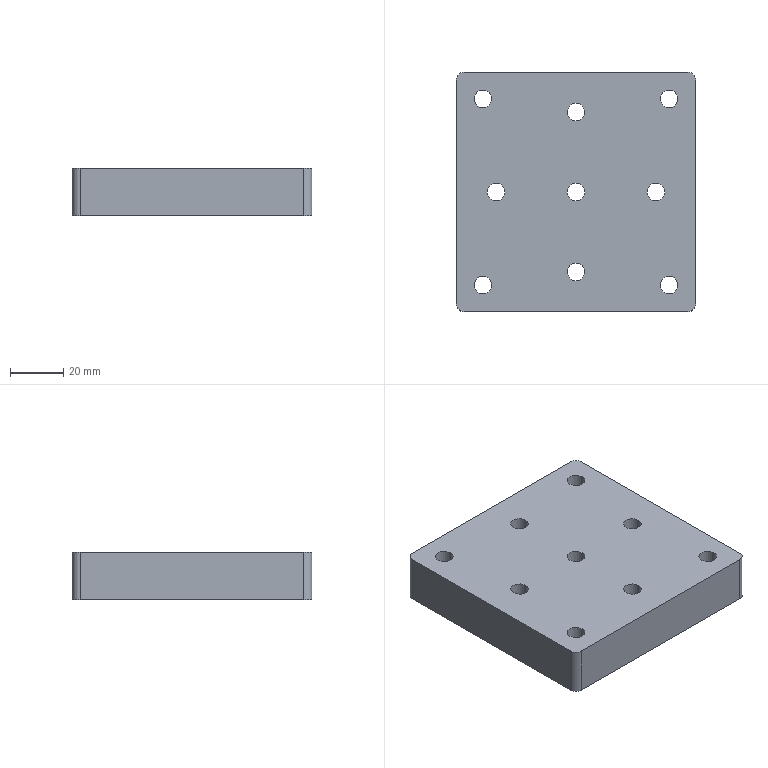Part | NX | features BREP 1 | 1 solid | 43 faces | box 90 x 90 x 18 mm | volume 136139 mm3 | cylinder 32 | plane 11 | commonest cylinder face diameters 6.6 x10 12 x10 6.647 x8 6 x4
STEP:
#1=CARTESIAN_POINT('',(6.,-30.,10.));
#2=VERTEX_POINT('',#1);
#3=CARTESIAN_POINT('',(-6.,-30.,10.));
#4=VERTEX_POINT('',#3);
#5=CARTESIAN_POINT('',(0.,-30.,10.));
#6=DIRECTION('',(0.,0.,-1.));
#7=DIRECTION('',(1.,0.,0.));
#8=AXIS2_PLACEMENT_3D('',#5,#6,#7);
#9=CIRCLE('',#8,6.);
#10=EDGE_CURVE('',#2,#4,#9,.T.);
#11=ORIENTED_EDGE('',*,*,#10,.T.);
#12=CARTESIAN_POINT('',(0.,-30.,10.));
#13=DIRECTION('',(0.,0.,-1.));
#14=DIRECTION('',(-1.,0.,0.));
#15=AXIS2_PLACEMENT_3D('',#12,#13,#14);
#16=CIRCLE('',#15,6.);
#17=EDGE_CURVE('',#4,#2,#16,.T.);
#18=ORIENTED_EDGE('',*,*,#17,.T.);
#19=EDGE_LOOP('',(#11,#18));
#20=FACE_BOUND('',#19,.T.);
#21=CARTESIAN_POINT('',(3.3,-30.,10.));
#22=VERTEX_POINT('',#21);
#23=CARTESIAN_POINT('',(-3.3,-30.,10.));
#24=VERTEX_POINT('',#23);
#25=CARTESIAN_POINT('',(0.,-30.,10.));
#26=DIRECTION('',(0.,0.,1.));
#27=DIRECTION('',(1.,0.,0.));
#28=AXIS2_PLACEMENT_3D('',#25,#26,#27);
#29=CIRCLE('',#28,3.3);
#30=EDGE_CURVE('',#22,#24,#29,.T.);
#31=ORIENTED_EDGE('',*,*,#30,.T.);
#32=CARTESIAN_POINT('',(0.,-30.,10.));
#33=DIRECTION('',(0.,0.,1.));
#34=DIRECTION('',(-1.,0.,0.));
#35=AXIS2_PLACEMENT_3D('',#32,#33,#34);
#36=CIRCLE('',#35,3.3);
#37=EDGE_CURVE('',#24,#22,#36,.T.);
#38=ORIENTED_EDGE('',*,*,#37,.T.);
#39=EDGE_LOOP('',(#31,#38));
#40=FACE_BOUND('',#39,.T.);
#41=CARTESIAN_POINT('',(3.3,-30.,10.));
#42=DIRECTION('',(0.,0.,1.));
#43=DIRECTION('',(1.,0.,0.));
#44=AXIS2_PLACEMENT_3D('',#41,#42,#43);
#45=PLANE('',#44);
#46=ADVANCED_FACE('',(#20,#40),#45,.F.);
#47=CARTESIAN_POINT('',(6.,-30.,0.));
#48=VERTEX_POINT('',#47);
#49=CARTESIAN_POINT('',(6.,-30.,0.));
#50=DIRECTION('',(0.,0.,1.));
#51=VECTOR('',#50,1000.);
#52=LINE('',#49,#51);
#53=EDGE_CURVE('',#2,#48,#52,.F.);
#54=ORIENTED_EDGE('',*,*,#53,.F.);
#55=ORIENTED_EDGE('',*,*,#17,.F.);
#56=CARTESIAN_POINT('',(-6.,-30.,0.));
#57=VERTEX_POINT('',#56);
#58=CARTESIAN_POINT('',(-6.,-30.,0.));
#59=DIRECTION('',(0.,0.,1.));
#60=VECTOR('',#59,1000.);
#61=LINE('',#58,#60);
#62=EDGE_CURVE('',#4,#57,#61,.F.);
#63=ORIENTED_EDGE('',*,*,#62,.T.);
#64=CARTESIAN_POINT('',(0.,-30.,0.));
#65=DIRECTION('',(0.,0.,1.));
#66=DIRECTION('',(1.,0.,0.));
#67=AXIS2_PLACEMENT_3D('',#64,#65,#66);
#68=CIRCLE('',#67,6.);
#69=EDGE_CURVE('',#48,#57,#68,.T.);
#70=ORIENTED_EDGE('',*,*,#69,.F.);
#71=EDGE_LOOP('',(#54,#55,#63,#70));
#72=FACE_BOUND('',#71,.T.);
#73=CARTESIAN_POINT('',(0.,-30.,0.));
#74=DIRECTION('',(0.,0.,1.));
#75=DIRECTION('',(-1.,0.,0.));
#76=AXIS2_PLACEMENT_3D('',#73,#74,#75);
#77=CYLINDRICAL_SURFACE('',#76,6.);
#78=ADVANCED_FACE('',(#72),#77,.F.);
#79=CARTESIAN_POINT('',(-42.,45.,0.));
#80=VERTEX_POINT('',#79);
#81=CARTESIAN_POINT('',(42.,45.,0.));
#82=VERTEX_POINT('',#81);
#83=CARTESIAN_POINT('',(-42.,45.,0.));
#84=DIRECTION('',(1.,0.,0.));
#85=VECTOR('',#84,1000.);
#86=LINE('',#83,#85);
#87=EDGE_CURVE('',#80,#82,#86,.T.);
#88=ORIENTED_EDGE('',*,*,#87,.T.);
#89=CARTESIAN_POINT('',(45.,42.,0.));
#90=VERTEX_POINT('',#89);
#91=CARTESIAN_POINT('',(42.,42.,0.));
#92=DIRECTION('',(0.,0.,-1.));
#93=DIRECTION('',(0.,1.,0.));
#94=AXIS2_PLACEMENT_3D('',#91,#92,#93);
#95=CIRCLE('',#94,3.);
#96=EDGE_CURVE('',#82,#90,#95,.T.);
#97=ORIENTED_EDGE('',*,*,#96,.T.);
#98=CARTESIAN_POINT('',(45.,-42.,0.));
#99=VERTEX_POINT('',#98);
#100=CARTESIAN_POINT('',(45.,42.,0.));
#101=DIRECTION('',(0.,-1.,0.));
#102=VECTOR('',#101,1000.);
#103=LINE('',#100,#102);
#104=EDGE_CURVE('',#90,#99,#103,.T.);
#105=ORIENTED_EDGE('',*,*,#104,.T.);
#106=CARTESIAN_POINT('',(42.,-45.,0.));
#107=VERTEX_POINT('',#106);
#108=CARTESIAN_POINT('',(42.,-42.,0.));
#109=DIRECTION('',(0.,0.,-1.));
#110=DIRECTION('',(1.,0.,0.));
#111=AXIS2_PLACEMENT_3D('',#108,#109,#110);
#112=CIRCLE('',#111,3.);
#113=EDGE_CURVE('',#99,#107,#112,.T.);
#114=ORIENTED_EDGE('',*,*,#113,.T.);
#115=CARTESIAN_POINT('',(-42.,-45.,0.));
#116=VERTEX_POINT('',#115);
#117=CARTESIAN_POINT('',(42.,-45.,0.));
#118=DIRECTION('',(-1.,0.,0.));
#119=VECTOR('',#118,1000.);
#120=LINE('',#117,#119);
#121=EDGE_CURVE('',#107,#116,#120,.T.);
#122=ORIENTED_EDGE('',*,*,#121,.T.);
#123=CARTESIAN_POINT('',(-45.,-42.,0.));
#124=VERTEX_POINT('',#123);
#125=CARTESIAN_POINT('',(-42.,-42.,0.));
#126=DIRECTION('',(0.,0.,-1.));
#127=DIRECTION('',(0.,-1.,0.));
#128=AXIS2_PLACEMENT_3D('',#125,#126,#127);
#129=CIRCLE('',#128,3.);
#130=EDGE_CURVE('',#116,#124,#129,.T.);
#131=ORIENTED_EDGE('',*,*,#130,.T.);
#132=CARTESIAN_POINT('',(-45.,42.,0.));
#133=VERTEX_POINT('',#132);
#134=CARTESIAN_POINT('',(-45.,-42.,0.));
#135=DIRECTION('',(0.,1.,0.));
#136=VECTOR('',#135,1000.);
#137=LINE('',#134,#136);
#138=EDGE_CURVE('',#124,#133,#137,.T.);
#139=ORIENTED_EDGE('',*,*,#138,.T.);
#140=CARTESIAN_POINT('',(-42.,42.,0.));
#141=DIRECTION('',(0.,0.,-1.));
#142=DIRECTION('',(-1.,0.,0.));
#143=AXIS2_PLACEMENT_3D('',#140,#141,#142);
#144=CIRCLE('',#143,3.);
#145=EDGE_CURVE('',#133,#80,#144,.T.);
#146=ORIENTED_EDGE('',*,*,#145,.T.);
#147=EDGE_LOOP('',(#88,#97,#105,#114,#122,#131,#139,#146));
#148=FACE_BOUND('',#147,.T.);
#149=CARTESIAN_POINT('',(-6.,0.,0.));
#150=VERTEX_POINT('',#149);
#151=CARTESIAN_POINT('',(6.,0.,0.));
#152=VERTEX_POINT('',#151);
#153=CARTESIAN_POINT('',(0.,0.,0.));
#154=DIRECTION('',(0.,0.,1.));
#155=DIRECTION('',(-1.,0.,0.));
#156=AXIS2_PLACEMENT_3D('',#153,#154,#155);
#157=CIRCLE('',#156,6.);
#158=EDGE_CURVE('',#150,#152,#157,.T.);
#159=ORIENTED_EDGE('',*,*,#158,.T.);
#160=CARTESIAN_POINT('',(0.,0.,0.));
#161=DIRECTION('',(0.,0.,1.));
#162=DIRECTION('',(1.,0.,0.));
#163=AXIS2_PLACEMENT_3D('',#160,#161,#162);
#164=CIRCLE('',#163,6.);
#165=EDGE_CURVE('',#152,#150,#164,.T.);
#166=ORIENTED_EDGE('',*,*,#165,.T.);
#167=EDGE_LOOP('',(#159,#166));
#168=FACE_BOUND('',#167,.T.);
#169=ORIENTED_EDGE('',*,*,#69,.T.);
#170=CARTESIAN_POINT('',(0.,-30.,0.));
#171=DIRECTION('',(0.,0.,1.));
#172=DIRECTION('',(-1.,0.,0.));
#173=AXIS2_PLACEMENT_3D('',#170,#171,#172);
#174=CIRCLE('',#173,6.);
#175=EDGE_CURVE('',#57,#48,#174,.T.);
#176=ORIENTED_EDGE('',*,*,#175,.T.);
#177=EDGE_LOOP('',(#169,#176));
#178=FACE_BOUND('',#177,.T.);
#179=CARTESIAN_POINT('',(-31.677,35.,0.));
#180=VERTEX_POINT('',#179);
#181=CARTESIAN_POINT('',(-38.324,35.,0.));
#182=VERTEX_POINT('',#181);
#183=CARTESIAN_POINT('',(-35.,35.,0.));
#184=DIRECTION('',(0.,0.,1.));
#185=DIRECTION('',(1.,0.,0.));
#186=AXIS2_PLACEMENT_3D('',#183,#184,#185);
#187=CIRCLE('',#186,3.324);
#188=EDGE_CURVE('',#180,#182,#187,.T.);
#189=ORIENTED_EDGE('',*,*,#188,.T.);
#190=CARTESIAN_POINT('',(-35.,35.,0.));
#191=DIRECTION('',(0.,0.,1.));
#192=DIRECTION('',(-1.,0.,0.));
#193=AXIS2_PLACEMENT_3D('',#190,#191,#192);
#194=CIRCLE('',#193,3.324);
#195=EDGE_CURVE('',#182,#180,#194,.T.);
#196=ORIENTED_EDGE('',*,*,#195,.T.);
#197=EDGE_LOOP('',(#189,#196));
#198=FACE_BOUND('',#197,.T.);
#199=CARTESIAN_POINT('',(-38.324,-35.,0.));
#200=VERTEX_POINT('',#199);
#201=CARTESIAN_POINT('',(-31.677,-35.,0.));
#202=VERTEX_POINT('',#201);
#203=CARTESIAN_POINT('',(-35.,-35.,0.));
#204=DIRECTION('',(0.,0.,1.));
#205=DIRECTION('',(-1.,0.,0.));
#206=AXIS2_PLACEMENT_3D('',#203,#204,#205);
#207=CIRCLE('',#206,3.324);
#208=EDGE_CURVE('',#200,#202,#207,.T.);
#209=ORIENTED_EDGE('',*,*,#208,.T.);
#210=CARTESIAN_POINT('',(-35.,-35.,0.));
#211=DIRECTION('',(0.,0.,1.));
#212=DIRECTION('',(1.,0.,0.));
#213=AXIS2_PLACEMENT_3D('',#210,#211,#212);
#214=CIRCLE('',#213,3.324);
#215=EDGE_CURVE('',#202,#200,#214,.T.);
#216=ORIENTED_EDGE('',*,*,#215,.T.);
#217=EDGE_LOOP('',(#209,#216));
#218=FACE_BOUND('',#217,.T.);
#219=CARTESIAN_POINT('',(31.677,35.,0.));
#220=VERTEX_POINT('',#219);
#221=CARTESIAN_POINT('',(38.324,35.,0.));
#222=VERTEX_POINT('',#221);
#223=CARTESIAN_POINT('',(35.,35.,0.));
#224=DIRECTION('',(0.,0.,1.));
#225=DIRECTION('',(-1.,0.,0.));
#226=AXIS2_PLACEMENT_3D('',#223,#224,#225);
#227=CIRCLE('',#226,3.324);
#228=EDGE_CURVE('',#220,#222,#227,.T.);
#229=ORIENTED_EDGE('',*,*,#228,.T.);
#230=CARTESIAN_POINT('',(35.,35.,0.));
#231=DIRECTION('',(0.,0.,1.));
#232=DIRECTION('',(1.,0.,0.));
#233=AXIS2_PLACEMENT_3D('',#230,#231,#232);
#234=CIRCLE('',#233,3.324);
#235=EDGE_CURVE('',#222,#220,#234,.T.);
#236=ORIENTED_EDGE('',*,*,#235,.T.);
#237=EDGE_LOOP('',(#229,#236));
#238=FACE_BOUND('',#237,.T.);
#239=CARTESIAN_POINT('',(31.677,-35.,0.));
#240=VERTEX_POINT('',#239);
#241=CARTESIAN_POINT('',(38.324,-35.,0.));
#242=VERTEX_POINT('',#241);
#243=CARTESIAN_POINT('',(35.,-35.,0.));
#244=DIRECTION('',(0.,0.,1.));
#245=DIRECTION('',(-1.,0.,0.));
#246=AXIS2_PLACEMENT_3D('',#243,#244,#245);
#247=CIRCLE('',#246,3.324);
#248=EDGE_CURVE('',#240,#242,#247,.T.);
#249=ORIENTED_EDGE('',*,*,#248,.T.);
#250=CARTESIAN_POINT('',(35.,-35.,0.));
#251=DIRECTION('',(0.,0.,1.));
#252=DIRECTION('',(1.,0.,0.));
#253=AXIS2_PLACEMENT_3D('',#250,#251,#252);
#254=CIRCLE('',#253,3.324);
#255=EDGE_CURVE('',#242,#240,#254,.T.);
#256=ORIENTED_EDGE('',*,*,#255,.T.);
#257=EDGE_LOOP('',(#249,#256));
#258=FACE_BOUND('',#257,.T.);
#259=CARTESIAN_POINT('',(-36.,0.,0.));
#260=VERTEX_POINT('',#259);
#261=CARTESIAN_POINT('',(-24.,0.,0.));
#262=VERTEX_POINT('',#261);
#263=CARTESIAN_POINT('',(-30.,0.,0.));
#264=DIRECTION('',(0.,0.,1.));
#265=DIRECTION('',(-1.,0.,0.));
#266=AXIS2_PLACEMENT_3D('',#263,#264,#265);
#267=CIRCLE('',#266,6.);
#268=EDGE_CURVE('',#260,#262,#267,.T.);
#269=ORIENTED_EDGE('',*,*,#268,.T.);
#270=CARTESIAN_POINT('',(-30.,0.,0.));
#271=DIRECTION('',(0.,0.,1.));
#272=DIRECTION('',(1.,0.,0.));
#273=AXIS2_PLACEMENT_3D('',#270,#271,#272);
#274=CIRCLE('',#273,6.);
#275=EDGE_CURVE('',#262,#260,#274,.T.);
#276=ORIENTED_EDGE('',*,*,#275,.T.);
#277=EDGE_LOOP('',(#269,#276));
#278=FACE_BOUND('',#277,.T.);
#279=CARTESIAN_POINT('',(24.,0.,0.));
#280=VERTEX_POINT('',#279);
#281=CARTESIAN_POINT('',(36.,0.,0.));
#282=VERTEX_POINT('',#281);
#283=CARTESIAN_POINT('',(30.,0.,0.));
#284=DIRECTION('',(0.,0.,1.));
#285=DIRECTION('',(-1.,0.,0.));
#286=AXIS2_PLACEMENT_3D('',#283,#284,#285);
#287=CIRCLE('',#286,6.);
#288=EDGE_CURVE('',#280,#282,#287,.T.);
#289=ORIENTED_EDGE('',*,*,#288,.T.);
#290=CARTESIAN_POINT('',(30.,0.,0.));
#291=DIRECTION('',(0.,0.,1.));
#292=DIRECTION('',(1.,0.,0.));
#293=AXIS2_PLACEMENT_3D('',#290,#291,#292);
#294=CIRCLE('',#293,6.);
#295=EDGE_CURVE('',#282,#280,#294,.T.);
#296=ORIENTED_EDGE('',*,*,#295,.T.);
#297=EDGE_LOOP('',(#289,#296));
#298=FACE_BOUND('',#297,.T.);
#299=CARTESIAN_POINT('',(-6.,30.,0.));
#300=VERTEX_POINT('',#299);
#301=CARTESIAN_POINT('',(6.,30.,0.));
#302=VERTEX_POINT('',#301);
#303=CARTESIAN_POINT('',(0.,30.,0.));
#304=DIRECTION('',(0.,0.,1.));
#305=DIRECTION('',(-1.,0.,0.));
#306=AXIS2_PLACEMENT_3D('',#303,#304,#305);
#307=CIRCLE('',#306,6.);
#308=EDGE_CURVE('',#300,#302,#307,.T.);
#309=ORIENTED_EDGE('',*,*,#308,.T.);
#310=CARTESIAN_POINT('',(0.,30.,0.));
#311=DIRECTION('',(0.,0.,1.));
#312=DIRECTION('',(1.,0.,0.));
#313=AXIS2_PLACEMENT_3D('',#310,#311,#312);
#314=CIRCLE('',#313,6.);
#315=EDGE_CURVE('',#302,#300,#314,.T.);
#316=ORIENTED_EDGE('',*,*,#315,.T.);
#317=EDGE_LOOP('',(#309,#316));
#318=FACE_BOUND('',#317,.T.);
#319=CARTESIAN_POINT('',(0.,0.,0.));
#320=DIRECTION('',(0.,0.,1.));
#321=DIRECTION('',(1.,0.,0.));
#322=AXIS2_PLACEMENT_3D('',#319,#320,#321);
#323=PLANE('',#322);
#324=ADVANCED_FACE('',(#148,#168,#178,#198,#218,#238,#258,#278,#298,#318),#323,.F.);
#325=CARTESIAN_POINT('',(-42.,45.,18.));
#326=VERTEX_POINT('',#325);
#327=CARTESIAN_POINT('',(-42.,45.,18.));
#328=DIRECTION('',(0.,0.,-1.));
#329=VECTOR('',#328,1000.);
#330=LINE('',#327,#329);
#331=EDGE_CURVE('',#326,#80,#330,.T.);
#332=ORIENTED_EDGE('',*,*,#331,.T.);
#333=ORIENTED_EDGE('',*,*,#145,.F.);
#334=CARTESIAN_POINT('',(-45.,42.,18.));
#335=VERTEX_POINT('',#334);
#336=CARTESIAN_POINT('',(-45.,42.,0.));
#337=DIRECTION('',(0.,0.,1.));
#338=VECTOR('',#337,1000.);
#339=LINE('',#336,#338);
#340=EDGE_CURVE('',#133,#335,#339,.T.);
#341=ORIENTED_EDGE('',*,*,#340,.T.);
#342=CARTESIAN_POINT('',(-42.,42.,18.));
#343=DIRECTION('',(0.,0.,1.));
#344=DIRECTION('',(0.,1.,0.));
#345=AXIS2_PLACEMENT_3D('',#342,#343,#344);
#346=CIRCLE('',#345,3.);
#347=EDGE_CURVE('',#326,#335,#346,.T.);
#348=ORIENTED_EDGE('',*,*,#347,.F.);
#349=EDGE_LOOP('',(#332,#333,#341,#348));
#350=FACE_BOUND('',#349,.T.);
#351=CARTESIAN_POINT('',(-42.,42.,9.));
#352=DIRECTION('',(0.,0.,1.));
#353=DIRECTION('',(0.,1.,0.));
#354=AXIS2_PLACEMENT_3D('',#351,#352,#353);
#355=CYLINDRICAL_SURFACE('',#354,3.);
#356=ADVANCED_FACE('',(#350),#355,.T.);
#357=CARTESIAN_POINT('',(-45.,-42.,18.));
#358=VERTEX_POINT('',#357);
#359=CARTESIAN_POINT('',(-42.,-45.,18.));
#360=VERTEX_POINT('',#359);
#361=CARTESIAN_POINT('',(-42.,-42.,18.));
#362=DIRECTION('',(0.,0.,1.));
#363=DIRECTION('',(-1.,0.,0.));
#364=AXIS2_PLACEMENT_3D('',#361,#362,#363);
#365=CIRCLE('',#364,3.);
#366=EDGE_CURVE('',#358,#360,#365,.T.);
#367=ORIENTED_EDGE('',*,*,#366,.T.);
#368=CARTESIAN_POINT('',(42.,-45.,18.));
#369=VERTEX_POINT('',#368);
#370=CARTESIAN_POINT('',(42.,-45.,18.));
#371=DIRECTION('',(-1.,0.,0.));
#372=VECTOR('',#371,1000.);
#373=LINE('',#370,#372);
#374=EDGE_CURVE('',#369,#360,#373,.T.);
#375=ORIENTED_EDGE('',*,*,#374,.F.);
#376=CARTESIAN_POINT('',(45.,-42.,18.));
#377=VERTEX_POINT('',#376);
#378=CARTESIAN_POINT('',(42.,-42.,18.));
#379=DIRECTION('',(0.,0.,1.));
#380=DIRECTION('',(0.,-1.,0.));
#381=AXIS2_PLACEMENT_3D('',#378,#379,#380);
#382=CIRCLE('',#381,3.);
#383=EDGE_CURVE('',#369,#377,#382,.T.);
#384=ORIENTED_EDGE('',*,*,#383,.T.);
#385=CARTESIAN_POINT('',(45.,42.,18.));
#386=VERTEX_POINT('',#385);
#387=CARTESIAN_POINT('',(45.,42.,18.));
#388=DIRECTION('',(0.,-1.,0.));
#389=VECTOR('',#388,1000.);
#390=LINE('',#387,#389);
#391=EDGE_CURVE('',#386,#377,#390,.T.);
#392=ORIENTED_EDGE('',*,*,#391,.F.);
#393=CARTESIAN_POINT('',(42.,45.,18.));
#394=VERTEX_POINT('',#393);
#395=CARTESIAN_POINT('',(42.,42.,18.));
#396=DIRECTION('',(0.,0.,1.));
#397=DIRECTION('',(1.,0.,0.));
#398=AXIS2_PLACEMENT_3D('',#395,#396,#397);
#399=CIRCLE('',#398,3.);
#400=EDGE_CURVE('',#386,#394,#399,.T.);
#401=ORIENTED_EDGE('',*,*,#400,.T.);
#402=CARTESIAN_POINT('',(-42.,45.,18.));
#403=DIRECTION('',(1.,0.,0.));
#404=VECTOR('',#403,1000.);
#405=LINE('',#402,#404);
#406=EDGE_CURVE('',#326,#394,#405,.T.);
#407=ORIENTED_EDGE('',*,*,#406,.F.);
#408=ORIENTED_EDGE('',*,*,#347,.T.);
#409=CARTESIAN_POINT('',(-45.,-42.,18.));
#410=DIRECTION('',(0.,1.,0.));
#411=VECTOR('',#410,1000.);
#412=LINE('',#409,#411);
#413=EDGE_CURVE('',#358,#335,#412,.T.);
#414=ORIENTED_EDGE('',*,*,#413,.F.);
#415=EDGE_LOOP('',(#367,#375,#384,#392,#401,#407,#408,#414));
#416=FACE_BOUND('',#415,.T.);
#417=CARTESIAN_POINT('',(-3.3,0.,18.));
#418=VERTEX_POINT('',#417);
#419=CARTESIAN_POINT('',(3.3,0.,18.));
#420=VERTEX_POINT('',#419);
#421=CARTESIAN_POINT('',(0.,0.,18.));
#422=DIRECTION('',(0.,0.,-1.));
#423=DIRECTION('',(-1.,0.,0.));
#424=AXIS2_PLACEMENT_3D('',#421,#422,#423);
#425=CIRCLE('',#424,3.3);
#426=EDGE_CURVE('',#418,#420,#425,.T.);
#427=ORIENTED_EDGE('',*,*,#426,.T.);
#428=CARTESIAN_POINT('',(0.,0.,18.));
#429=DIRECTION('',(0.,0.,-1.));
#430=DIRECTION('',(1.,0.,0.));
#431=AXIS2_PLACEMENT_3D('',#428,#429,#430);
#432=CIRCLE('',#431,3.3);
#433=EDGE_CURVE('',#420,#418,#432,.T.);
#434=ORIENTED_EDGE('',*,*,#433,.T.);
#435=EDGE_LOOP('',(#427,#434));
#436=FACE_BOUND('',#435,.T.);
#437=CARTESIAN_POINT('',(3.3,-30.,18.));
#438=VERTEX_POINT('',#437);
#439=CARTESIAN_POINT('',(-3.3,-30.,18.));
#440=VERTEX_POINT('',#439);
#441=CARTESIAN_POINT('',(0.,-30.,18.));
#442=DIRECTION('',(0.,0.,-1.));
#443=DIRECTION('',(1.,0.,0.));
#444=AXIS2_PLACEMENT_3D('',#441,#442,#443);
#445=CIRCLE('',#444,3.3);
#446=EDGE_CURVE('',#438,#440,#445,.T.);
#447=ORIENTED_EDGE('',*,*,#446,.T.);
#448=CARTESIAN_POINT('',(0.,-30.,18.));
#449=DIRECTION('',(0.,0.,-1.));
#450=DIRECTION('',(-1.,0.,0.));
#451=AXIS2_PLACEMENT_3D('',#448,#449,#450);
#452=CIRCLE('',#451,3.3);
#453=EDGE_CURVE('',#440,#438,#452,.T.);
#454=ORIENTED_EDGE('',*,*,#453,.T.);
#455=EDGE_LOOP('',(#447,#454));
#456=FACE_BOUND('',#455,.T.);
#457=CARTESIAN_POINT('',(-31.677,35.,18.));
#458=VERTEX_POINT('',#457);
#459=CARTESIAN_POINT('',(-38.324,35.,18.));
#460=VERTEX_POINT('',#459);
#461=CARTESIAN_POINT('',(-35.,35.,18.));
#462=DIRECTION('',(0.,0.,-1.));
#463=DIRECTION('',(1.,0.,0.));
#464=AXIS2_PLACEMENT_3D('',#461,#462,#463);
#465=CIRCLE('',#464,3.324);
#466=EDGE_CURVE('',#458,#460,#465,.T.);
#467=ORIENTED_EDGE('',*,*,#466,.T.);
#468=CARTESIAN_POINT('',(-35.,35.,18.));
#469=DIRECTION('',(0.,0.,-1.));
#470=DIRECTION('',(-1.,0.,0.));
#471=AXIS2_PLACEMENT_3D('',#468,#469,#470);
#472=CIRCLE('',#471,3.324);
#473=EDGE_CURVE('',#460,#458,#472,.T.);
#474=ORIENTED_EDGE('',*,*,#473,.T.);
#475=EDGE_LOOP('',(#467,#474));
#476=FACE_BOUND('',#475,.T.);
#477=CARTESIAN_POINT('',(-38.324,-35.,18.));
#478=VERTEX_POINT('',#477);
#479=CARTESIAN_POINT('',(-31.677,-35.,18.));
#480=VERTEX_POINT('',#479);
#481=CARTESIAN_POINT('',(-35.,-35.,18.));
#482=DIRECTION('',(0.,0.,-1.));
#483=DIRECTION('',(-1.,0.,0.));
#484=AXIS2_PLACEMENT_3D('',#481,#482,#483);
#485=CIRCLE('',#484,3.324);
#486=EDGE_CURVE('',#478,#480,#485,.T.);
#487=ORIENTED_EDGE('',*,*,#486,.T.);
#488=CARTESIAN_POINT('',(-35.,-35.,18.));
#489=DIRECTION('',(0.,0.,-1.));
#490=DIRECTION('',(1.,0.,0.));
#491=AXIS2_PLACEMENT_3D('',#488,#489,#490);
#492=CIRCLE('',#491,3.324);
#493=EDGE_CURVE('',#480,#478,#492,.T.);
#494=ORIENTED_EDGE('',*,*,#493,.T.);
#495=EDGE_LOOP('',(#487,#494));
#496=FACE_BOUND('',#495,.T.);
#497=CARTESIAN_POINT('',(31.677,35.,18.));
#498=VERTEX_POINT('',#497);
#499=CARTESIAN_POINT('',(38.324,35.,18.));
#500=VERTEX_POINT('',#499);
#501=CARTESIAN_POINT('',(35.,35.,18.));
#502=DIRECTION('',(0.,0.,-1.));
#503=DIRECTION('',(-1.,0.,0.));
#504=AXIS2_PLACEMENT_3D('',#501,#502,#503);
#505=CIRCLE('',#504,3.324);
#506=EDGE_CURVE('',#498,#500,#505,.T.);
#507=ORIENTED_EDGE('',*,*,#506,.T.);
#508=CARTESIAN_POINT('',(35.,35.,18.));
#509=DIRECTION('',(0.,0.,-1.));
#510=DIRECTION('',(1.,0.,0.));
#511=AXIS2_PLACEMENT_3D('',#508,#509,#510);
#512=CIRCLE('',#511,3.324);
#513=EDGE_CURVE('',#500,#498,#512,.T.);
#514=ORIENTED_EDGE('',*,*,#513,.T.);
#515=EDGE_LOOP('',(#507,#514));
#516=FACE_BOUND('',#515,.T.);
#517=CARTESIAN_POINT('',(31.677,-35.,18.));
#518=VERTEX_POINT('',#517);
#519=CARTESIAN_POINT('',(38.324,-35.,18.));
#520=VERTEX_POINT('',#519);
#521=CARTESIAN_POINT('',(35.,-35.,18.));
#522=DIRECTION('',(0.,0.,-1.));
#523=DIRECTION('',(-1.,0.,0.));
#524=AXIS2_PLACEMENT_3D('',#521,#522,#523);
#525=CIRCLE('',#524,3.324);
#526=EDGE_CURVE('',#518,#520,#525,.T.);
#527=ORIENTED_EDGE('',*,*,#526,.T.);
#528=CARTESIAN_POINT('',(35.,-35.,18.));
#529=DIRECTION('',(0.,0.,-1.));
#530=DIRECTION('',(1.,0.,0.));
#531=AXIS2_PLACEMENT_3D('',#528,#529,#530);
#532=CIRCLE('',#531,3.324);
#533=EDGE_CURVE('',#520,#518,#532,.T.);
#534=ORIENTED_EDGE('',*,*,#533,.T.);
#535=EDGE_LOOP('',(#527,#534));
#536=FACE_BOUND('',#535,.T.);
#537=CARTESIAN_POINT('',(-33.3,0.,18.));
#538=VERTEX_POINT('',#537);
#539=CARTESIAN_POINT('',(-26.7,0.,18.));
#540=VERTEX_POINT('',#539);
#541=CARTESIAN_POINT('',(-30.,0.,18.));
#542=DIRECTION('',(0.,0.,-1.));
#543=DIRECTION('',(-1.,0.,0.));
#544=AXIS2_PLACEMENT_3D('',#541,#542,#543);
#545=CIRCLE('',#544,3.3);
#546=EDGE_CURVE('',#538,#540,#545,.T.);
#547=ORIENTED_EDGE('',*,*,#546,.T.);
#548=CARTESIAN_POINT('',(-30.,0.,18.));
#549=DIRECTION('',(0.,0.,-1.));
#550=DIRECTION('',(1.,0.,0.));
#551=AXIS2_PLACEMENT_3D('',#548,#549,#550);
#552=CIRCLE('',#551,3.3);
#553=EDGE_CURVE('',#540,#538,#552,.T.);
#554=ORIENTED_EDGE('',*,*,#553,.T.);
#555=EDGE_LOOP('',(#547,#554));
#556=FACE_BOUND('',#555,.T.);
#557=CARTESIAN_POINT('',(26.7,0.,18.));
#558=VERTEX_POINT('',#557);
#559=CARTESIAN_POINT('',(33.3,0.,18.));
#560=VERTEX_POINT('',#559);
#561=CARTESIAN_POINT('',(30.,0.,18.));
#562=DIRECTION('',(0.,0.,-1.));
#563=DIRECTION('',(-1.,0.,0.));
#564=AXIS2_PLACEMENT_3D('',#561,#562,#563);
#565=CIRCLE('',#564,3.3);
#566=EDGE_CURVE('',#558,#560,#565,.T.);
#567=ORIENTED_EDGE('',*,*,#566,.T.);
#568=CARTESIAN_POINT('',(30.,0.,18.));
#569=DIRECTION('',(0.,0.,-1.));
#570=DIRECTION('',(1.,0.,0.));
#571=AXIS2_PLACEMENT_3D('',#568,#569,#570);
#572=CIRCLE('',#571,3.3);
#573=EDGE_CURVE('',#560,#558,#572,.T.);
#574=ORIENTED_EDGE('',*,*,#573,.T.);
#575=EDGE_LOOP('',(#567,#574));
#576=FACE_BOUND('',#575,.T.);
#577=CARTESIAN_POINT('',(-3.3,30.,18.));
#578=VERTEX_POINT('',#577);
#579=CARTESIAN_POINT('',(3.3,30.,18.));
#580=VERTEX_POINT('',#579);
#581=CARTESIAN_POINT('',(0.,30.,18.));
#582=DIRECTION('',(0.,0.,-1.));
#583=DIRECTION('',(-1.,0.,0.));
#584=AXIS2_PLACEMENT_3D('',#581,#582,#583);
#585=CIRCLE('',#584,3.3);
#586=EDGE_CURVE('',#578,#580,#585,.T.);
#587=ORIENTED_EDGE('',*,*,#586,.T.);
#588=CARTESIAN_POINT('',(0.,30.,18.));
#589=DIRECTION('',(0.,0.,-1.));
#590=DIRECTION('',(1.,0.,0.));
#591=AXIS2_PLACEMENT_3D('',#588,#589,#590);
#592=CIRCLE('',#591,3.3);
#593=EDGE_CURVE('',#580,#578,#592,.T.);
#594=ORIENTED_EDGE('',*,*,#593,.T.);
#595=EDGE_LOOP('',(#587,#594));
#596=FACE_BOUND('',#595,.T.);
#597=CARTESIAN_POINT('',(0.,0.,18.));
#598=DIRECTION('',(0.,0.,1.));
#599=DIRECTION('',(1.,0.,0.));
#600=AXIS2_PLACEMENT_3D('',#597,#598,#599);
#601=PLANE('',#600);
#602=ADVANCED_FACE('',(#416,#436,#456,#476,#496,#516,#536,#556,#576,#596),#601,.T.);
#603=ORIENTED_EDGE('',*,*,#138,.F.);
#604=CARTESIAN_POINT('',(-45.,-42.,18.));
#605=DIRECTION('',(0.,0.,-1.));
#606=VECTOR('',#605,1000.);
#607=LINE('',#604,#606);
#608=EDGE_CURVE('',#358,#124,#607,.T.);
#609=ORIENTED_EDGE('',*,*,#608,.F.);
#610=ORIENTED_EDGE('',*,*,#413,.T.);
#611=ORIENTED_EDGE('',*,*,#340,.F.);
#612=EDGE_LOOP('',(#603,#609,#610,#611));
#613=FACE_BOUND('',#612,.T.);
#614=CARTESIAN_POINT('',(-45.,-45.,0.));
#615=DIRECTION('',(1.,0.,0.));
#616=DIRECTION('',(0.,1.,0.));
#617=AXIS2_PLACEMENT_3D('',#614,#615,#616);
#618=PLANE('',#617);
#619=ADVANCED_FACE('',(#613),#618,.F.);
#620=ORIENTED_EDGE('',*,*,#608,.T.);
#621=ORIENTED_EDGE('',*,*,#130,.F.);
#622=CARTESIAN_POINT('',(-42.,-45.,0.));
#623=DIRECTION('',(0.,0.,1.));
#624=VECTOR('',#623,1000.);
#625=LINE('',#622,#624);
#626=EDGE_CURVE('',#116,#360,#625,.T.);
#627=ORIENTED_EDGE('',*,*,#626,.T.);
#628=ORIENTED_EDGE('',*,*,#366,.F.);
#629=EDGE_LOOP('',(#620,#621,#627,#628));
#630=FACE_BOUND('',#629,.T.);
#631=CARTESIAN_POINT('',(-42.,-42.,9.));
#632=DIRECTION('',(0.,0.,1.));
#633=DIRECTION('',(-1.,0.,0.));
#634=AXIS2_PLACEMENT_3D('',#631,#632,#633);
#635=CYLINDRICAL_SURFACE('',#634,3.);
#636=ADVANCED_FACE('',(#630),#635,.T.);
#637=ORIENTED_EDGE('',*,*,#121,.F.);
#638=CARTESIAN_POINT('',(42.,-45.,18.));
#639=DIRECTION('',(0.,0.,-1.));
#640=VECTOR('',#639,1000.);
#641=LINE('',#638,#640);
#642=EDGE_CURVE('',#369,#107,#641,.T.);
#643=ORIENTED_EDGE('',*,*,#642,.F.);
#644=ORIENTED_EDGE('',*,*,#374,.T.);
#645=ORIENTED_EDGE('',*,*,#626,.F.);
#646=EDGE_LOOP('',(#637,#643,#644,#645));
#647=FACE_BOUND('',#646,.T.);
#648=CARTESIAN_POINT('',(45.,-45.,0.));
#649=DIRECTION('',(0.,1.,0.));
#650=DIRECTION('',(1.,0.,0.));
#651=AXIS2_PLACEMENT_3D('',#648,#649,#650);
#652=PLANE('',#651);
#653=ADVANCED_FACE('',(#647),#652,.F.);
#654=ORIENTED_EDGE('',*,*,#642,.T.);
#655=ORIENTED_EDGE('',*,*,#113,.F.);
#656=CARTESIAN_POINT('',(45.,-42.,0.));
#657=DIRECTION('',(0.,0.,1.));
#658=VECTOR('',#657,1000.);
#659=LINE('',#656,#658);
#660=EDGE_CURVE('',#99,#377,#659,.T.);
#661=ORIENTED_EDGE('',*,*,#660,.T.);
#662=ORIENTED_EDGE('',*,*,#383,.F.);
#663=EDGE_LOOP('',(#654,#655,#661,#662));
#664=FACE_BOUND('',#663,.T.);
#665=CARTESIAN_POINT('',(42.,-42.,9.));
#666=DIRECTION('',(0.,0.,1.));
#667=DIRECTION('',(0.,-1.,0.));
#668=AXIS2_PLACEMENT_3D('',#665,#666,#667);
#669=CYLINDRICAL_SURFACE('',#668,3.);
#670=ADVANCED_FACE('',(#664),#669,.T.);
#671=ORIENTED_EDGE('',*,*,#104,.F.);
#672=CARTESIAN_POINT('',(45.,42.,18.));
#673=DIRECTION('',(0.,0.,-1.));
#674=VECTOR('',#673,1000.);
#675=LINE('',#672,#674);
#676=EDGE_CURVE('',#386,#90,#675,.T.);
#677=ORIENTED_EDGE('',*,*,#676,.F.);
#678=ORIENTED_EDGE('',*,*,#391,.T.);
#679=ORIENTED_EDGE('',*,*,#660,.F.);
#680=EDGE_LOOP('',(#671,#677,#678,#679));
#681=FACE_BOUND('',#680,.T.);
#682=CARTESIAN_POINT('',(45.,45.,0.));
#683=DIRECTION('',(-1.,0.,0.));
#684=DIRECTION('',(0.,0.,1.));
#685=AXIS2_PLACEMENT_3D('',#682,#683,#684);
#686=PLANE('',#685);
#687=ADVANCED_FACE('',(#681),#686,.F.);
#688=ORIENTED_EDGE('',*,*,#676,.T.);
#689=ORIENTED_EDGE('',*,*,#96,.F.);
#690=CARTESIAN_POINT('',(42.,45.,0.));
#691=DIRECTION('',(0.,0.,1.));
#692=VECTOR('',#691,1000.);
#693=LINE('',#690,#692);
#694=EDGE_CURVE('',#82,#394,#693,.T.);
#695=ORIENTED_EDGE('',*,*,#694,.T.);
#696=ORIENTED_EDGE('',*,*,#400,.F.);
#697=EDGE_LOOP('',(#688,#689,#695,#696));
#698=FACE_BOUND('',#697,.T.);
#699=CARTESIAN_POINT('',(42.,42.,9.));
#700=DIRECTION('',(0.,0.,1.));
#701=DIRECTION('',(1.,0.,0.));
#702=AXIS2_PLACEMENT_3D('',#699,#700,#701);
#703=CYLINDRICAL_SURFACE('',#702,3.);
#704=ADVANCED_FACE('',(#698),#703,.T.);
#705=ORIENTED_EDGE('',*,*,#406,.T.);
#706=ORIENTED_EDGE('',*,*,#694,.F.);
#707=ORIENTED_EDGE('',*,*,#87,.F.);
#708=ORIENTED_EDGE('',*,*,#331,.F.);
#709=EDGE_LOOP('',(#705,#706,#707,#708));
#710=FACE_BOUND('',#709,.T.);
#711=CARTESIAN_POINT('',(-45.,45.,0.));
#712=DIRECTION('',(0.,-1.,0.));
#713=DIRECTION('',(0.,0.,-1.));
#714=AXIS2_PLACEMENT_3D('',#711,#712,#713);
#715=PLANE('',#714);
#716=ADVANCED_FACE('',(#710),#715,.F.);
#717=CARTESIAN_POINT('',(3.3,0.,10.));
#718=VERTEX_POINT('',#717);
#719=CARTESIAN_POINT('',(3.3,0.,10.));
#720=DIRECTION('',(0.,0.,1.));
#721=VECTOR('',#720,1000.);
#722=LINE('',#719,#721);
#723=EDGE_CURVE('',#420,#718,#722,.F.);
#724=ORIENTED_EDGE('',*,*,#723,.T.);
#725=CARTESIAN_POINT('',(-3.3,0.,10.));
#726=VERTEX_POINT('',#725);
#727=CARTESIAN_POINT('',(0.,0.,10.));
#728=DIRECTION('',(0.,0.,1.));
#729=DIRECTION('',(-1.,0.,0.));
#730=AXIS2_PLACEMENT_3D('',#727,#728,#729);
#731=CIRCLE('',#730,3.3);
#732=EDGE_CURVE('',#726,#718,#731,.T.);
#733=ORIENTED_EDGE('',*,*,#732,.F.);
#734=CARTESIAN_POINT('',(-3.3,0.,10.));
#735=DIRECTION('',(0.,0.,1.));
#736=VECTOR('',#735,1000.);
#737=LINE('',#734,#736);
#738=EDGE_CURVE('',#418,#726,#737,.F.);
#739=ORIENTED_EDGE('',*,*,#738,.F.);
#740=ORIENTED_EDGE('',*,*,#433,.F.);
#741=EDGE_LOOP('',(#724,#733,#739,#740));
#742=FACE_BOUND('',#741,.T.);
#743=CARTESIAN_POINT('',(0.,0.,0.));
#744=DIRECTION('',(0.,0.,1.));
#745=DIRECTION('',(1.,0.,0.));
#746=AXIS2_PLACEMENT_3D('',#743,#744,#745);
#747=CYLINDRICAL_SURFACE('',#746,3.3);
#748=ADVANCED_FACE('',(#742),#747,.F.);
#749=ORIENTED_EDGE('',*,*,#738,.T.);
#750=CARTESIAN_POINT('',(0.,0.,10.));
#751=DIRECTION('',(0.,0.,1.));
#752=DIRECTION('',(1.,0.,0.));
#753=AXIS2_PLACEMENT_3D('',#750,#751,#752);
#754=CIRCLE('',#753,3.3);
#755=EDGE_CURVE('',#718,#726,#754,.T.);
#756=ORIENTED_EDGE('',*,*,#755,.F.);
#757=ORIENTED_EDGE('',*,*,#723,.F.);
#758=ORIENTED_EDGE('',*,*,#426,.F.);
#759=EDGE_LOOP('',(#749,#756,#757,#758));
#760=FACE_BOUND('',#759,.T.);
#761=CARTESIAN_POINT('',(0.,0.,0.));
#762=DIRECTION('',(0.,0.,1.));
#763=DIRECTION('',(1.,0.,0.));
#764=AXIS2_PLACEMENT_3D('',#761,#762,#763);
#765=CYLINDRICAL_SURFACE('',#764,3.3);
#766=ADVANCED_FACE('',(#760),#765,.F.);
#767=CARTESIAN_POINT('',(6.,0.,10.));
#768=VERTEX_POINT('',#767);
#769=CARTESIAN_POINT('',(-6.,0.,10.));
#770=VERTEX_POINT('',#769);
#771=CARTESIAN_POINT('',(0.,0.,10.));
#772=DIRECTION('',(0.,0.,-1.));
#773=DIRECTION('',(1.,0.,0.));
#774=AXIS2_PLACEMENT_3D('',#771,#772,#773);
#775=CIRCLE('',#774,6.);
#776=EDGE_CURVE('',#768,#770,#775,.T.);
#777=ORIENTED_EDGE('',*,*,#776,.T.);
#778=CARTESIAN_POINT('',(0.,0.,10.));
#779=DIRECTION('',(0.,0.,-1.));
#780=DIRECTION('',(-1.,0.,0.));
#781=AXIS2_PLACEMENT_3D('',#778,#779,#780);
#782=CIRCLE('',#781,6.);
#783=EDGE_CURVE('',#770,#768,#782,.T.);
#784=ORIENTED_EDGE('',*,*,#783,.T.);
#785=EDGE_LOOP('',(#777,#784));
#786=FACE_BOUND('',#785,.T.);
#787=ORIENTED_EDGE('',*,*,#755,.T.);
#788=ORIENTED_EDGE('',*,*,#732,.T.);
#789=EDGE_LOOP('',(#787,#788));
#790=FACE_BOUND('',#789,.T.);
#791=CARTESIAN_POINT('',(3.3,-30.,10.));
#792=DIRECTION('',(0.,0.,1.));
#793=DIRECTION('',(1.,0.,0.));
#794=AXIS2_PLACEMENT_3D('',#791,#792,#793);
#795=PLANE('',#794);
#796=ADVANCED_FACE('',(#786,#790),#795,.F.);
#797=CARTESIAN_POINT('',(6.,0.,0.));
#798=DIRECTION('',(0.,0.,1.));
#799=VECTOR('',#798,1000.);
#800=LINE('',#797,#799);
#801=EDGE_CURVE('',#768,#152,#800,.F.);
#802=ORIENTED_EDGE('',*,*,#801,.F.);
#803=ORIENTED_EDGE('',*,*,#783,.F.);
#804=CARTESIAN_POINT('',(-6.,0.,0.));
#805=DIRECTION('',(0.,0.,1.));
#806=VECTOR('',#805,1000.);
#807=LINE('',#804,#806);
#808=EDGE_CURVE('',#770,#150,#807,.F.);
#809=ORIENTED_EDGE('',*,*,#808,.T.);
#810=ORIENTED_EDGE('',*,*,#165,.F.);
#811=EDGE_LOOP('',(#802,#803,#809,#810));
#812=FACE_BOUND('',#811,.T.);
#813=CARTESIAN_POINT('',(0.,0.,0.));
#814=DIRECTION('',(0.,0.,1.));
#815=DIRECTION('',(1.,0.,0.));
#816=AXIS2_PLACEMENT_3D('',#813,#814,#815);
#817=CYLINDRICAL_SURFACE('',#816,6.);
#818=ADVANCED_FACE('',(#812),#817,.F.);
#819=ORIENTED_EDGE('',*,*,#808,.F.);
#820=ORIENTED_EDGE('',*,*,#776,.F.);
#821=ORIENTED_EDGE('',*,*,#801,.T.);
#822=ORIENTED_EDGE('',*,*,#158,.F.);
#823=EDGE_LOOP('',(#819,#820,#821,#822));
#824=FACE_BOUND('',#823,.T.);
#825=CARTESIAN_POINT('',(0.,0.,0.));
#826=DIRECTION('',(0.,0.,1.));
#827=DIRECTION('',(1.,0.,0.));
#828=AXIS2_PLACEMENT_3D('',#825,#826,#827);
#829=CYLINDRICAL_SURFACE('',#828,6.);
#830=ADVANCED_FACE('',(#824),#829,.F.);
#831=CARTESIAN_POINT('',(-3.3,-30.,10.));
#832=DIRECTION('',(0.,0.,1.));
#833=VECTOR('',#832,1000.);
#834=LINE('',#831,#833);
#835=EDGE_CURVE('',#24,#440,#834,.T.);
#836=ORIENTED_EDGE('',*,*,#835,.F.);
#837=ORIENTED_EDGE('',*,*,#30,.F.);
#838=CARTESIAN_POINT('',(3.3,-30.,10.));
#839=DIRECTION('',(0.,0.,1.));
#840=VECTOR('',#839,1000.);
#841=LINE('',#838,#840);
#842=EDGE_CURVE('',#22,#438,#841,.T.);
#843=ORIENTED_EDGE('',*,*,#842,.T.);
#844=ORIENTED_EDGE('',*,*,#453,.F.);
#845=EDGE_LOOP('',(#836,#837,#843,#844));
#846=FACE_BOUND('',#845,.T.);
#847=CARTESIAN_POINT('',(0.,-30.,0.));
#848=DIRECTION('',(0.,0.,1.));
#849=DIRECTION('',(-1.,0.,0.));
#850=AXIS2_PLACEMENT_3D('',#847,#848,#849);
#851=CYLINDRICAL_SURFACE('',#850,3.3);
#852=ADVANCED_FACE('',(#846),#851,.F.);
#853=ORIENTED_EDGE('',*,*,#842,.F.);
#854=ORIENTED_EDGE('',*,*,#37,.F.);
#855=ORIENTED_EDGE('',*,*,#835,.T.);
#856=ORIENTED_EDGE('',*,*,#446,.F.);
#857=EDGE_LOOP('',(#853,#854,#855,#856));
#858=FACE_BOUND('',#857,.T.);
#859=CARTESIAN_POINT('',(0.,-30.,0.));
#860=DIRECTION('',(0.,0.,1.));
#861=DIRECTION('',(-1.,0.,0.));
#862=AXIS2_PLACEMENT_3D('',#859,#860,#861);
#863=CYLINDRICAL_SURFACE('',#862,3.3);
#864=ADVANCED_FACE('',(#858),#863,.F.);
#865=ORIENTED_EDGE('',*,*,#473,.F.);
#866=CARTESIAN_POINT('',(-38.324,35.,0.));
#867=DIRECTION('',(0.,0.,1.));
#868=VECTOR('',#867,1000.);
#869=LINE('',#866,#868);
#870=EDGE_CURVE('',#182,#460,#869,.T.);
#871=ORIENTED_EDGE('',*,*,#870,.F.);
#872=ORIENTED_EDGE('',*,*,#188,.F.);
#873=CARTESIAN_POINT('',(-31.677,35.,0.));
#874=DIRECTION('',(0.,0.,1.));
#875=VECTOR('',#874,1000.);
#876=LINE('',#873,#875);
#877=EDGE_CURVE('',#180,#458,#876,.T.);
#878=ORIENTED_EDGE('',*,*,#877,.T.);
#879=EDGE_LOOP('',(#865,#871,#872,#878));
#880=FACE_BOUND('',#879,.T.);
#881=CARTESIAN_POINT('',(-35.,35.,0.));
#882=DIRECTION('',(0.,0.,1.));
#883=DIRECTION('',(1.,0.,0.));
#884=AXIS2_PLACEMENT_3D('',#881,#882,#883);
#885=CYLINDRICAL_SURFACE('',#884,3.324);
#886=ADVANCED_FACE('',(#880),#885,.F.);
#887=ORIENTED_EDGE('',*,*,#466,.F.);
#888=ORIENTED_EDGE('',*,*,#877,.F.);
#889=ORIENTED_EDGE('',*,*,#195,.F.);
#890=ORIENTED_EDGE('',*,*,#870,.T.);
#891=EDGE_LOOP('',(#887,#888,#889,#890));
#892=FACE_BOUND('',#891,.T.);
#893=CARTESIAN_POINT('',(-35.,35.,0.));
#894=DIRECTION('',(0.,0.,1.));
#895=DIRECTION('',(1.,0.,0.));
#896=AXIS2_PLACEMENT_3D('',#893,#894,#895);
#897=CYLINDRICAL_SURFACE('',#896,3.324);
#898=ADVANCED_FACE('',(#892),#897,.F.);
#899=ORIENTED_EDGE('',*,*,#493,.F.);
#900=CARTESIAN_POINT('',(-31.677,-35.,0.));
#901=DIRECTION('',(0.,0.,1.));
#902=VECTOR('',#901,1000.);
#903=LINE('',#900,#902);
#904=EDGE_CURVE('',#480,#202,#903,.F.);
#905=ORIENTED_EDGE('',*,*,#904,.T.);
#906=ORIENTED_EDGE('',*,*,#208,.F.);
#907=CARTESIAN_POINT('',(-38.324,-35.,0.));
#908=DIRECTION('',(0.,0.,1.));
#909=VECTOR('',#908,1000.);
#910=LINE('',#907,#909);
#911=EDGE_CURVE('',#478,#200,#910,.F.);
#912=ORIENTED_EDGE('',*,*,#911,.F.);
#913=EDGE_LOOP('',(#899,#905,#906,#912));
#914=FACE_BOUND('',#913,.T.);
#915=CARTESIAN_POINT('',(-35.,-35.,0.));
#916=DIRECTION('',(0.,0.,1.));
#917=DIRECTION('',(-1.,0.,0.));
#918=AXIS2_PLACEMENT_3D('',#915,#916,#917);
#919=CYLINDRICAL_SURFACE('',#918,3.324);
#920=ADVANCED_FACE('',(#914),#919,.F.);
#921=ORIENTED_EDGE('',*,*,#486,.F.);
#922=ORIENTED_EDGE('',*,*,#911,.T.);
#923=ORIENTED_EDGE('',*,*,#215,.F.);
#924=ORIENTED_EDGE('',*,*,#904,.F.);
#925=EDGE_LOOP('',(#921,#922,#923,#924));
#926=FACE_BOUND('',#925,.T.);
#927=CARTESIAN_POINT('',(-35.,-35.,0.));
#928=DIRECTION('',(0.,0.,1.));
#929=DIRECTION('',(-1.,0.,0.));
#930=AXIS2_PLACEMENT_3D('',#927,#928,#929);
#931=CYLINDRICAL_SURFACE('',#930,3.324);
#932=ADVANCED_FACE('',(#926),#931,.F.);
#933=ORIENTED_EDGE('',*,*,#513,.F.);
#934=CARTESIAN_POINT('',(38.324,35.,0.));
#935=DIRECTION('',(0.,0.,1.));
#936=VECTOR('',#935,1000.);
#937=LINE('',#934,#936);
#938=EDGE_CURVE('',#500,#222,#937,.F.);
#939=ORIENTED_EDGE('',*,*,#938,.T.);
#940=ORIENTED_EDGE('',*,*,#228,.F.);
#941=CARTESIAN_POINT('',(31.677,35.,0.));
#942=DIRECTION('',(0.,0.,1.));
#943=VECTOR('',#942,1000.);
#944=LINE('',#941,#943);
#945=EDGE_CURVE('',#498,#220,#944,.F.);
#946=ORIENTED_EDGE('',*,*,#945,.F.);
#947=EDGE_LOOP('',(#933,#939,#940,#946));
#948=FACE_BOUND('',#947,.T.);
#949=CARTESIAN_POINT('',(35.,35.,0.));
#950=DIRECTION('',(0.,0.,1.));
#951=DIRECTION('',(-1.,0.,0.));
#952=AXIS2_PLACEMENT_3D('',#949,#950,#951);
#953=CYLINDRICAL_SURFACE('',#952,3.324);
#954=ADVANCED_FACE('',(#948),#953,.F.);
#955=ORIENTED_EDGE('',*,*,#506,.F.);
#956=ORIENTED_EDGE('',*,*,#945,.T.);
#957=ORIENTED_EDGE('',*,*,#235,.F.);
#958=ORIENTED_EDGE('',*,*,#938,.F.);
#959=EDGE_LOOP('',(#955,#956,#957,#958));
#960=FACE_BOUND('',#959,.T.);
#961=CARTESIAN_POINT('',(35.,35.,0.));
#962=DIRECTION('',(0.,0.,1.));
#963=DIRECTION('',(-1.,0.,0.));
#964=AXIS2_PLACEMENT_3D('',#961,#962,#963);
#965=CYLINDRICAL_SURFACE('',#964,3.324);
#966=ADVANCED_FACE('',(#960),#965,.F.);
#967=ORIENTED_EDGE('',*,*,#533,.F.);
#968=CARTESIAN_POINT('',(38.324,-35.,0.));
#969=DIRECTION('',(0.,0.,1.));
#970=VECTOR('',#969,1000.);
#971=LINE('',#968,#970);
#972=EDGE_CURVE('',#520,#242,#971,.F.);
#973=ORIENTED_EDGE('',*,*,#972,.T.);
#974=ORIENTED_EDGE('',*,*,#248,.F.);
#975=CARTESIAN_POINT('',(31.677,-35.,0.));
#976=DIRECTION('',(0.,0.,1.));
#977=VECTOR('',#976,1000.);
#978=LINE('',#975,#977);
#979=EDGE_CURVE('',#518,#240,#978,.F.);
#980=ORIENTED_EDGE('',*,*,#979,.F.);
#981=EDGE_LOOP('',(#967,#973,#974,#980));
#982=FACE_BOUND('',#981,.T.);
#983=CARTESIAN_POINT('',(35.,-35.,0.));
#984=DIRECTION('',(0.,0.,1.));
#985=DIRECTION('',(-1.,0.,0.));
#986=AXIS2_PLACEMENT_3D('',#983,#984,#985);
#987=CYLINDRICAL_SURFACE('',#986,3.324);
#988=ADVANCED_FACE('',(#982),#987,.F.);
#989=ORIENTED_EDGE('',*,*,#526,.F.);
#990=ORIENTED_EDGE('',*,*,#979,.T.);
#991=ORIENTED_EDGE('',*,*,#255,.F.);
#992=ORIENTED_EDGE('',*,*,#972,.F.);
#993=EDGE_LOOP('',(#989,#990,#991,#992));
#994=FACE_BOUND('',#993,.T.);
#995=CARTESIAN_POINT('',(35.,-35.,0.));
#996=DIRECTION('',(0.,0.,1.));
#997=DIRECTION('',(-1.,0.,0.));
#998=AXIS2_PLACEMENT_3D('',#995,#996,#997);
#999=CYLINDRICAL_SURFACE('',#998,3.324);
#1000=ADVANCED_FACE('',(#994),#999,.F.);
#1001=CARTESIAN_POINT('',(-26.7,0.,10.));
#1002=VERTEX_POINT('',#1001);
#1003=CARTESIAN_POINT('',(-26.7,0.,10.));
#1004=DIRECTION('',(0.,0.,1.));
#1005=VECTOR('',#1004,1000.);
#1006=LINE('',#1003,#1005);
#1007=EDGE_CURVE('',#540,#1002,#1006,.F.);
#1008=ORIENTED_EDGE('',*,*,#1007,.T.);
#1009=CARTESIAN_POINT('',(-33.3,0.,10.));
#1010=VERTEX_POINT('',#1009);
#1011=CARTESIAN_POINT('',(-30.,0.,10.));
#1012=DIRECTION('',(0.,0.,1.));
#1013=DIRECTION('',(-1.,0.,0.));
#1014=AXIS2_PLACEMENT_3D('',#1011,#1012,#1013);
#1015=CIRCLE('',#1014,3.3);
#1016=EDGE_CURVE('',#1010,#1002,#1015,.T.);
#1017=ORIENTED_EDGE('',*,*,#1016,.F.);
#1018=CARTESIAN_POINT('',(-33.3,0.,10.));
#1019=DIRECTION('',(0.,0.,1.));
#1020=VECTOR('',#1019,1000.);
#1021=LINE('',#1018,#1020);
#1022=EDGE_CURVE('',#538,#1010,#1021,.F.);
#1023=ORIENTED_EDGE('',*,*,#1022,.F.);
#1024=ORIENTED_EDGE('',*,*,#553,.F.);
#1025=EDGE_LOOP('',(#1008,#1017,#1023,#1024));
#1026=FACE_BOUND('',#1025,.T.);
#1027=CARTESIAN_POINT('',(-30.,0.,0.));
#1028=DIRECTION('',(0.,0.,1.));
#1029=DIRECTION('',(1.,0.,0.));
#1030=AXIS2_PLACEMENT_3D('',#1027,#1028,#1029);
#1031=CYLINDRICAL_SURFACE('',#1030,3.3);
#1032=ADVANCED_FACE('',(#1026),#1031,.F.);
#1033=ORIENTED_EDGE('',*,*,#1022,.T.);
#1034=CARTESIAN_POINT('',(-30.,0.,10.));
#1035=DIRECTION('',(0.,0.,1.));
#1036=DIRECTION('',(1.,0.,0.));
#1037=AXIS2_PLACEMENT_3D('',#1034,#1035,#1036);
#1038=CIRCLE('',#1037,3.3);
#1039=EDGE_CURVE('',#1002,#1010,#1038,.T.);
#1040=ORIENTED_EDGE('',*,*,#1039,.F.);
#1041=ORIENTED_EDGE('',*,*,#1007,.F.);
#1042=ORIENTED_EDGE('',*,*,#546,.F.);
#1043=EDGE_LOOP('',(#1033,#1040,#1041,#1042));
#1044=FACE_BOUND('',#1043,.T.);
#1045=CARTESIAN_POINT('',(-30.,0.,0.));
#1046=DIRECTION('',(0.,0.,1.));
#1047=DIRECTION('',(1.,0.,0.));
#1048=AXIS2_PLACEMENT_3D('',#1045,#1046,#1047);
#1049=CYLINDRICAL_SURFACE('',#1048,3.3);
#1050=ADVANCED_FACE('',(#1044),#1049,.F.);
#1051=CARTESIAN_POINT('',(-24.,0.,10.));
#1052=VERTEX_POINT('',#1051);
#1053=CARTESIAN_POINT('',(-36.,0.,10.));
#1054=VERTEX_POINT('',#1053);
#1055=CARTESIAN_POINT('',(-30.,0.,10.));
#1056=DIRECTION('',(0.,0.,-1.));
#1057=DIRECTION('',(1.,0.,0.));
#1058=AXIS2_PLACEMENT_3D('',#1055,#1056,#1057);
#1059=CIRCLE('',#1058,6.);
#1060=EDGE_CURVE('',#1052,#1054,#1059,.T.);
#1061=ORIENTED_EDGE('',*,*,#1060,.T.);
#1062=CARTESIAN_POINT('',(-30.,0.,10.));
#1063=DIRECTION('',(0.,0.,-1.));
#1064=DIRECTION('',(-1.,0.,0.));
#1065=AXIS2_PLACEMENT_3D('',#1062,#1063,#1064);
#1066=CIRCLE('',#1065,6.);
#1067=EDGE_CURVE('',#1054,#1052,#1066,.T.);
#1068=ORIENTED_EDGE('',*,*,#1067,.T.);
#1069=EDGE_LOOP('',(#1061,#1068));
#1070=FACE_BOUND('',#1069,.T.);
#1071=ORIENTED_EDGE('',*,*,#1039,.T.);
#1072=ORIENTED_EDGE('',*,*,#1016,.T.);
#1073=EDGE_LOOP('',(#1071,#1072));
#1074=FACE_BOUND('',#1073,.T.);
#1075=CARTESIAN_POINT('',(3.3,-30.,10.));
#1076=DIRECTION('',(0.,0.,1.));
#1077=DIRECTION('',(1.,0.,0.));
#1078=AXIS2_PLACEMENT_3D('',#1075,#1076,#1077);
#1079=PLANE('',#1078);
#1080=ADVANCED_FACE('',(#1070,#1074),#1079,.F.);
#1081=CARTESIAN_POINT('',(-24.,0.,0.));
#1082=DIRECTION('',(0.,0.,1.));
#1083=VECTOR('',#1082,1000.);
#1084=LINE('',#1081,#1083);
#1085=EDGE_CURVE('',#1052,#262,#1084,.F.);
#1086=ORIENTED_EDGE('',*,*,#1085,.F.);
#1087=ORIENTED_EDGE('',*,*,#1067,.F.);
#1088=CARTESIAN_POINT('',(-36.,0.,0.));
#1089=DIRECTION('',(0.,0.,1.));
#1090=VECTOR('',#1089,1000.);
#1091=LINE('',#1088,#1090);
#1092=EDGE_CURVE('',#1054,#260,#1091,.F.);
#1093=ORIENTED_EDGE('',*,*,#1092,.T.);
#1094=ORIENTED_EDGE('',*,*,#275,.F.);
#1095=EDGE_LOOP('',(#1086,#1087,#1093,#1094));
#1096=FACE_BOUND('',#1095,.T.);
#1097=CARTESIAN_POINT('',(-30.,0.,0.));
#1098=DIRECTION('',(0.,0.,1.));
#1099=DIRECTION('',(1.,0.,0.));
#1100=AXIS2_PLACEMENT_3D('',#1097,#1098,#1099);
#1101=CYLINDRICAL_SURFACE('',#1100,6.);
#1102=ADVANCED_FACE('',(#1096),#1101,.F.);
#1103=ORIENTED_EDGE('',*,*,#1092,.F.);
#1104=ORIENTED_EDGE('',*,*,#1060,.F.);
#1105=ORIENTED_EDGE('',*,*,#1085,.T.);
#1106=ORIENTED_EDGE('',*,*,#268,.F.);
#1107=EDGE_LOOP('',(#1103,#1104,#1105,#1106));
#1108=FACE_BOUND('',#1107,.T.);
#1109=CARTESIAN_POINT('',(-30.,0.,0.));
#1110=DIRECTION('',(0.,0.,1.));
#1111=DIRECTION('',(1.,0.,0.));
#1112=AXIS2_PLACEMENT_3D('',#1109,#1110,#1111);
#1113=CYLINDRICAL_SURFACE('',#1112,6.);
#1114=ADVANCED_FACE('',(#1108),#1113,.F.);
#1115=CARTESIAN_POINT('',(33.3,0.,10.));
#1116=VERTEX_POINT('',#1115);
#1117=CARTESIAN_POINT('',(33.3,0.,10.));
#1118=DIRECTION('',(0.,0.,1.));
#1119=VECTOR('',#1118,1000.);
#1120=LINE('',#1117,#1119);
#1121=EDGE_CURVE('',#560,#1116,#1120,.F.);
#1122=ORIENTED_EDGE('',*,*,#1121,.T.);
#1123=CARTESIAN_POINT('',(26.7,0.,10.));
#1124=VERTEX_POINT('',#1123);
#1125=CARTESIAN_POINT('',(30.,0.,10.));
#1126=DIRECTION('',(0.,0.,1.));
#1127=DIRECTION('',(-1.,0.,0.));
#1128=AXIS2_PLACEMENT_3D('',#1125,#1126,#1127);
#1129=CIRCLE('',#1128,3.3);
#1130=EDGE_CURVE('',#1124,#1116,#1129,.T.);
#1131=ORIENTED_EDGE('',*,*,#1130,.F.);
#1132=CARTESIAN_POINT('',(26.7,0.,10.));
#1133=DIRECTION('',(0.,0.,1.));
#1134=VECTOR('',#1133,1000.);
#1135=LINE('',#1132,#1134);
#1136=EDGE_CURVE('',#558,#1124,#1135,.F.);
#1137=ORIENTED_EDGE('',*,*,#1136,.F.);
#1138=ORIENTED_EDGE('',*,*,#573,.F.);
#1139=EDGE_LOOP('',(#1122,#1131,#1137,#1138));
#1140=FACE_BOUND('',#1139,.T.);
#1141=CARTESIAN_POINT('',(30.,0.,0.));
#1142=DIRECTION('',(0.,0.,1.));
#1143=DIRECTION('',(1.,0.,0.));
#1144=AXIS2_PLACEMENT_3D('',#1141,#1142,#1143);
#1145=CYLINDRICAL_SURFACE('',#1144,3.3);
#1146=ADVANCED_FACE('',(#1140),#1145,.F.);
#1147=ORIENTED_EDGE('',*,*,#1136,.T.);
#1148=CARTESIAN_POINT('',(30.,0.,10.));
#1149=DIRECTION('',(0.,0.,1.));
#1150=DIRECTION('',(1.,0.,0.));
#1151=AXIS2_PLACEMENT_3D('',#1148,#1149,#1150);
#1152=CIRCLE('',#1151,3.3);
#1153=EDGE_CURVE('',#1116,#1124,#1152,.T.);
#1154=ORIENTED_EDGE('',*,*,#1153,.F.);
#1155=ORIENTED_EDGE('',*,*,#1121,.F.);
#1156=ORIENTED_EDGE('',*,*,#566,.F.);
#1157=EDGE_LOOP('',(#1147,#1154,#1155,#1156));
#1158=FACE_BOUND('',#1157,.T.);
#1159=CARTESIAN_POINT('',(30.,0.,0.));
#1160=DIRECTION('',(0.,0.,1.));
#1161=DIRECTION('',(1.,0.,0.));
#1162=AXIS2_PLACEMENT_3D('',#1159,#1160,#1161);
#1163=CYLINDRICAL_SURFACE('',#1162,3.3);
#1164=ADVANCED_FACE('',(#1158),#1163,.F.);
#1165=CARTESIAN_POINT('',(36.,0.,10.));
#1166=VERTEX_POINT('',#1165);
#1167=CARTESIAN_POINT('',(24.,0.,10.));
#1168=VERTEX_POINT('',#1167);
#1169=CARTESIAN_POINT('',(30.,0.,10.));
#1170=DIRECTION('',(0.,0.,-1.));
#1171=DIRECTION('',(1.,0.,0.));
#1172=AXIS2_PLACEMENT_3D('',#1169,#1170,#1171);
#1173=CIRCLE('',#1172,6.);
#1174=EDGE_CURVE('',#1166,#1168,#1173,.T.);
#1175=ORIENTED_EDGE('',*,*,#1174,.T.);
#1176=CARTESIAN_POINT('',(30.,0.,10.));
#1177=DIRECTION('',(0.,0.,-1.));
#1178=DIRECTION('',(-1.,0.,0.));
#1179=AXIS2_PLACEMENT_3D('',#1176,#1177,#1178);
#1180=CIRCLE('',#1179,6.);
#1181=EDGE_CURVE('',#1168,#1166,#1180,.T.);
#1182=ORIENTED_EDGE('',*,*,#1181,.T.);
#1183=EDGE_LOOP('',(#1175,#1182));
#1184=FACE_BOUND('',#1183,.T.);
#1185=ORIENTED_EDGE('',*,*,#1153,.T.);
#1186=ORIENTED_EDGE('',*,*,#1130,.T.);
#1187=EDGE_LOOP('',(#1185,#1186));
#1188=FACE_BOUND('',#1187,.T.);
#1189=CARTESIAN_POINT('',(3.3,-30.,10.));
#1190=DIRECTION('',(0.,0.,1.));
#1191=DIRECTION('',(1.,0.,0.));
#1192=AXIS2_PLACEMENT_3D('',#1189,#1190,#1191);
#1193=PLANE('',#1192);
#1194=ADVANCED_FACE('',(#1184,#1188),#1193,.F.);
#1195=CARTESIAN_POINT('',(36.,0.,0.));
#1196=DIRECTION('',(0.,0.,1.));
#1197=VECTOR('',#1196,1000.);
#1198=LINE('',#1195,#1197);
#1199=EDGE_CURVE('',#1166,#282,#1198,.F.);
#1200=ORIENTED_EDGE('',*,*,#1199,.F.);
#1201=ORIENTED_EDGE('',*,*,#1181,.F.);
#1202=CARTESIAN_POINT('',(24.,0.,0.));
#1203=DIRECTION('',(0.,0.,1.));
#1204=VECTOR('',#1203,1000.);
#1205=LINE('',#1202,#1204);
#1206=EDGE_CURVE('',#1168,#280,#1205,.F.);
#1207=ORIENTED_EDGE('',*,*,#1206,.T.);
#1208=ORIENTED_EDGE('',*,*,#295,.F.);
#1209=EDGE_LOOP('',(#1200,#1201,#1207,#1208));
#1210=FACE_BOUND('',#1209,.T.);
#1211=CARTESIAN_POINT('',(30.,0.,0.));
#1212=DIRECTION('',(0.,0.,1.));
#1213=DIRECTION('',(1.,0.,0.));
#1214=AXIS2_PLACEMENT_3D('',#1211,#1212,#1213);
#1215=CYLINDRICAL_SURFACE('',#1214,6.);
#1216=ADVANCED_FACE('',(#1210),#1215,.F.);
#1217=ORIENTED_EDGE('',*,*,#1206,.F.);
#1218=ORIENTED_EDGE('',*,*,#1174,.F.);
#1219=ORIENTED_EDGE('',*,*,#1199,.T.);
#1220=ORIENTED_EDGE('',*,*,#288,.F.);
#1221=EDGE_LOOP('',(#1217,#1218,#1219,#1220));
#1222=FACE_BOUND('',#1221,.T.);
#1223=CARTESIAN_POINT('',(30.,0.,0.));
#1224=DIRECTION('',(0.,0.,1.));
#1225=DIRECTION('',(1.,0.,0.));
#1226=AXIS2_PLACEMENT_3D('',#1223,#1224,#1225);
#1227=CYLINDRICAL_SURFACE('',#1226,6.);
#1228=ADVANCED_FACE('',(#1222),#1227,.F.);
#1229=CARTESIAN_POINT('',(3.3,30.,10.));
#1230=VERTEX_POINT('',#1229);
#1231=CARTESIAN_POINT('',(3.3,30.,10.));
#1232=DIRECTION('',(0.,0.,1.));
#1233=VECTOR('',#1232,1000.);
#1234=LINE('',#1231,#1233);
#1235=EDGE_CURVE('',#580,#1230,#1234,.F.);
#1236=ORIENTED_EDGE('',*,*,#1235,.T.);
#1237=CARTESIAN_POINT('',(-3.3,30.,10.));
#1238=VERTEX_POINT('',#1237);
#1239=CARTESIAN_POINT('',(0.,30.,10.));
#1240=DIRECTION('',(0.,0.,1.));
#1241=DIRECTION('',(-1.,0.,0.));
#1242=AXIS2_PLACEMENT_3D('',#1239,#1240,#1241);
#1243=CIRCLE('',#1242,3.3);
#1244=EDGE_CURVE('',#1238,#1230,#1243,.T.);
#1245=ORIENTED_EDGE('',*,*,#1244,.F.);
#1246=CARTESIAN_POINT('',(-3.3,30.,10.));
#1247=DIRECTION('',(0.,0.,1.));
#1248=VECTOR('',#1247,1000.);
#1249=LINE('',#1246,#1248);
#1250=EDGE_CURVE('',#578,#1238,#1249,.F.);
#1251=ORIENTED_EDGE('',*,*,#1250,.F.);
#1252=ORIENTED_EDGE('',*,*,#593,.F.);
#1253=EDGE_LOOP('',(#1236,#1245,#1251,#1252));
#1254=FACE_BOUND('',#1253,.T.);
#1255=CARTESIAN_POINT('',(0.,30.,0.));
#1256=DIRECTION('',(0.,0.,1.));
#1257=DIRECTION('',(1.,0.,0.));
#1258=AXIS2_PLACEMENT_3D('',#1255,#1256,#1257);
#1259=CYLINDRICAL_SURFACE('',#1258,3.3);
#1260=ADVANCED_FACE('',(#1254),#1259,.F.);
#1261=ORIENTED_EDGE('',*,*,#1250,.T.);
#1262=CARTESIAN_POINT('',(0.,30.,10.));
#1263=DIRECTION('',(0.,0.,1.));
#1264=DIRECTION('',(1.,0.,0.));
#1265=AXIS2_PLACEMENT_3D('',#1262,#1263,#1264);
#1266=CIRCLE('',#1265,3.3);
#1267=EDGE_CURVE('',#1230,#1238,#1266,.T.);
#1268=ORIENTED_EDGE('',*,*,#1267,.F.);
#1269=ORIENTED_EDGE('',*,*,#1235,.F.);
#1270=ORIENTED_EDGE('',*,*,#586,.F.);
#1271=EDGE_LOOP('',(#1261,#1268,#1269,#1270));
#1272=FACE_BOUND('',#1271,.T.);
#1273=CARTESIAN_POINT('',(0.,30.,0.));
#1274=DIRECTION('',(0.,0.,1.));
#1275=DIRECTION('',(1.,0.,0.));
#1276=AXIS2_PLACEMENT_3D('',#1273,#1274,#1275);
#1277=CYLINDRICAL_SURFACE('',#1276,3.3);
#1278=ADVANCED_FACE('',(#1272),#1277,.F.);
#1279=CARTESIAN_POINT('',(6.,30.,10.));
#1280=VERTEX_POINT('',#1279);
#1281=CARTESIAN_POINT('',(-6.,30.,10.));
#1282=VERTEX_POINT('',#1281);
#1283=CARTESIAN_POINT('',(0.,30.,10.));
#1284=DIRECTION('',(0.,0.,-1.));
#1285=DIRECTION('',(1.,0.,0.));
#1286=AXIS2_PLACEMENT_3D('',#1283,#1284,#1285);
#1287=CIRCLE('',#1286,6.);
#1288=EDGE_CURVE('',#1280,#1282,#1287,.T.);
#1289=ORIENTED_EDGE('',*,*,#1288,.T.);
#1290=CARTESIAN_POINT('',(0.,30.,10.));
#1291=DIRECTION('',(0.,0.,-1.));
#1292=DIRECTION('',(-1.,0.,0.));
#1293=AXIS2_PLACEMENT_3D('',#1290,#1291,#1292);
#1294=CIRCLE('',#1293,6.);
#1295=EDGE_CURVE('',#1282,#1280,#1294,.T.);
#1296=ORIENTED_EDGE('',*,*,#1295,.T.);
#1297=EDGE_LOOP('',(#1289,#1296));
#1298=FACE_BOUND('',#1297,.T.);
#1299=ORIENTED_EDGE('',*,*,#1267,.T.);
#1300=ORIENTED_EDGE('',*,*,#1244,.T.);
#1301=EDGE_LOOP('',(#1299,#1300));
#1302=FACE_BOUND('',#1301,.T.);
#1303=CARTESIAN_POINT('',(3.3,-30.,10.));
#1304=DIRECTION('',(0.,0.,1.));
#1305=DIRECTION('',(1.,0.,0.));
#1306=AXIS2_PLACEMENT_3D('',#1303,#1304,#1305);
#1307=PLANE('',#1306);
#1308=ADVANCED_FACE('',(#1298,#1302),#1307,.F.);
#1309=CARTESIAN_POINT('',(6.,30.,0.));
#1310=DIRECTION('',(0.,0.,1.));
#1311=VECTOR('',#1310,1000.);
#1312=LINE('',#1309,#1311);
#1313=EDGE_CURVE('',#1280,#302,#1312,.F.);
#1314=ORIENTED_EDGE('',*,*,#1313,.F.);
#1315=ORIENTED_EDGE('',*,*,#1295,.F.);
#1316=CARTESIAN_POINT('',(-6.,30.,0.));
#1317=DIRECTION('',(0.,0.,1.));
#1318=VECTOR('',#1317,1000.);
#1319=LINE('',#1316,#1318);
#1320=EDGE_CURVE('',#1282,#300,#1319,.F.);
#1321=ORIENTED_EDGE('',*,*,#1320,.T.);
#1322=ORIENTED_EDGE('',*,*,#315,.F.);
#1323=EDGE_LOOP('',(#1314,#1315,#1321,#1322));
#1324=FACE_BOUND('',#1323,.T.);
#1325=CARTESIAN_POINT('',(0.,30.,0.));
#1326=DIRECTION('',(0.,0.,1.));
#1327=DIRECTION('',(1.,0.,0.));
#1328=AXIS2_PLACEMENT_3D('',#1325,#1326,#1327);
#1329=CYLINDRICAL_SURFACE('',#1328,6.);
#1330=ADVANCED_FACE('',(#1324),#1329,.F.);
#1331=ORIENTED_EDGE('',*,*,#1320,.F.);
#1332=ORIENTED_EDGE('',*,*,#1288,.F.);
#1333=ORIENTED_EDGE('',*,*,#1313,.T.);
#1334=ORIENTED_EDGE('',*,*,#308,.F.);
#1335=EDGE_LOOP('',(#1331,#1332,#1333,#1334));
#1336=FACE_BOUND('',#1335,.T.);
#1337=CARTESIAN_POINT('',(0.,30.,0.));
#1338=DIRECTION('',(0.,0.,1.));
#1339=DIRECTION('',(1.,0.,0.));
#1340=AXIS2_PLACEMENT_3D('',#1337,#1338,#1339);
#1341=CYLINDRICAL_SURFACE('',#1340,6.);
#1342=ADVANCED_FACE('',(#1336),#1341,.F.);
#1343=ORIENTED_EDGE('',*,*,#62,.F.);
#1344=ORIENTED_EDGE('',*,*,#10,.F.);
#1345=ORIENTED_EDGE('',*,*,#53,.T.);
#1346=ORIENTED_EDGE('',*,*,#175,.F.);
#1347=EDGE_LOOP('',(#1343,#1344,#1345,#1346));
#1348=FACE_BOUND('',#1347,.T.);
#1349=CARTESIAN_POINT('',(0.,-30.,0.));
#1350=DIRECTION('',(0.,0.,1.));
#1351=DIRECTION('',(-1.,0.,0.));
#1352=AXIS2_PLACEMENT_3D('',#1349,#1350,#1351);
#1353=CYLINDRICAL_SURFACE('',#1352,6.);
#1354=ADVANCED_FACE('',(#1348),#1353,.F.);
#1355=CLOSED_SHELL('',(#46,#78,#324,#356,#602,#619,#636,#653,#670,#687,#704,#716,#748,#766,#796,#818,#830,#852,#864,#886,#898,#920,#932,#954,#966,#988,#1000,#1032,#1050,#1080,#1102,#1114,#1146,#1164,#1194,#1216,#1228,#1260,#1278,#1308,#1330,#1342,#1354));
#1356=MANIFOLD_SOLID_BREP('',#1355);
#1357=(LENGTH_UNIT()NAMED_UNIT(*)SI_UNIT(.MILLI.,.METRE.));
#1358=UNCERTAINTY_MEASURE_WITH_UNIT(LENGTH_MEASURE(0.00001),#1357,'','');
#1359=(NAMED_UNIT(*)PLANE_ANGLE_UNIT()SI_UNIT($,.RADIAN.));
#1360=(NAMED_UNIT(*)SI_UNIT($,.STERADIAN.)SOLID_ANGLE_UNIT());
#1361=(GEOMETRIC_REPRESENTATION_CONTEXT(3)GLOBAL_UNCERTAINTY_ASSIGNED_CONTEXT((#1358))GLOBAL_UNIT_ASSIGNED_CONTEXT((#1357,#1359,#1360))REPRESENTATION_CONTEXT('',''));
#1362=ADVANCED_BREP_SHAPE_REPRESENTATION('',(#1356),#1361);